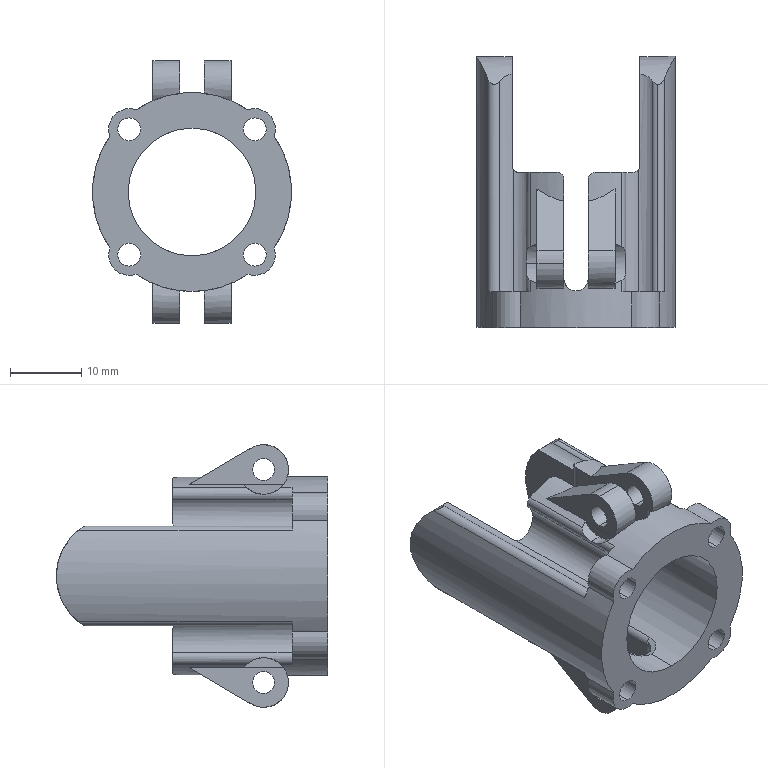Part | SolidWorks | features ICE 13, Fillet 7, MirrorPattern 4, Extrusion 1 | 1 solid | 128 faces | box 28 x 38.187 x 37 mm | volume 8059 mm3 | cylinder 75 | plane 31 | spline 14 | torus 4 | sphere 4 | commonest cylinder face diameters 2 x22 5.8 x12 7 x12 3.1 x8 3.2 x8 28 x7